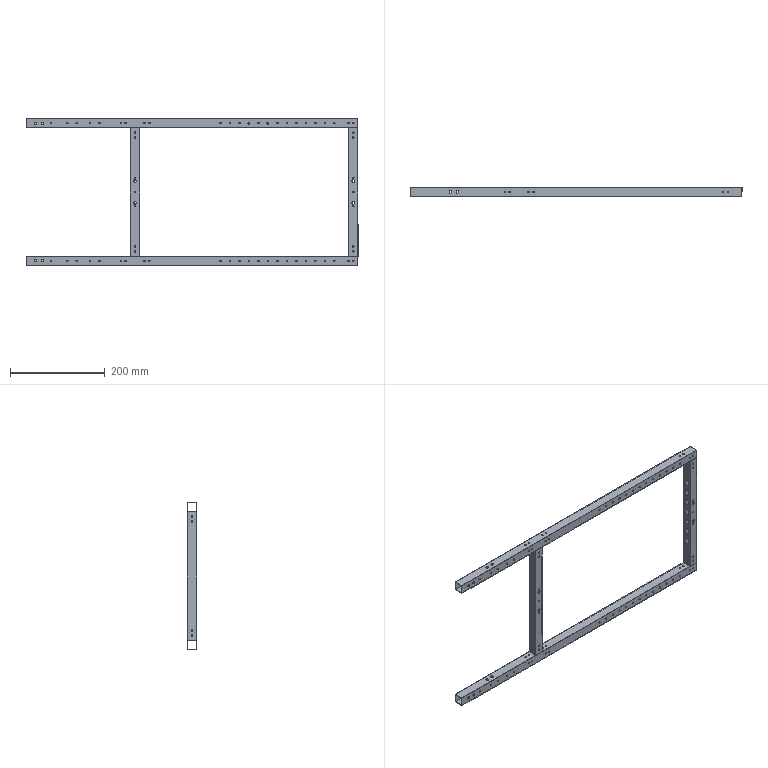Part | SolidWorks | features BaseBody 4 | 4 solids | 444 faces | box 700 x 20 x 310 mm | volume 144003 mm3 | cylinder 404 | plane 40 | commonest cylinder face diameters 3.2 x320 12 x28 5 x16 5.2 x16 5.5 x16 4 x8